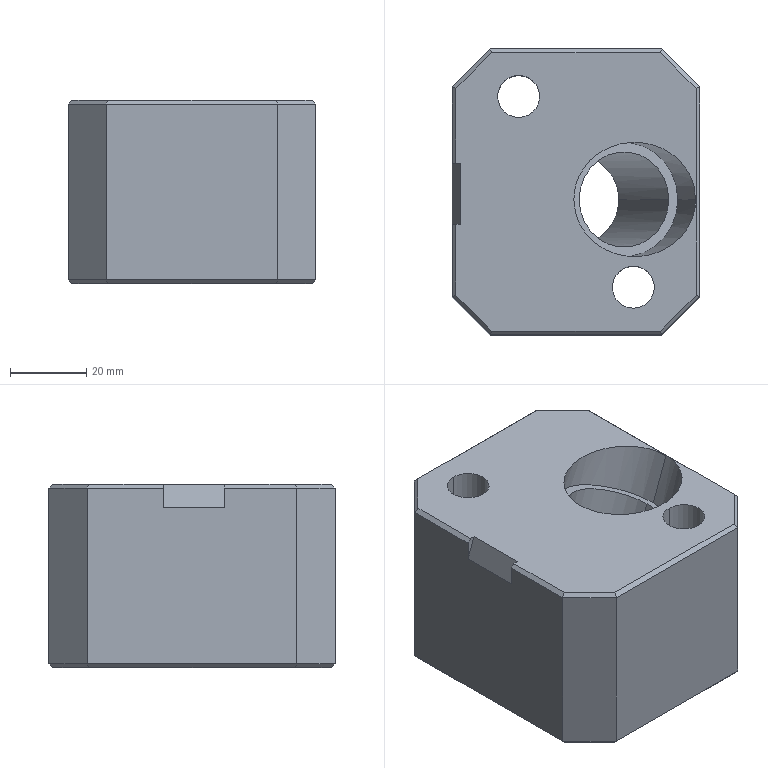Part | Creo | 1 solid | 49 faces | box 65 x 75 x 48 mm | volume 184557 mm3 | plane 33 | cylinder 16 | commonest cylinder face diameters 11 x4 18 x4 11.98 x2 12 x2 25 x2 30 x2
STEP:
#1=CARTESIAN_POINT('',(-250.936,-112.003,0.9999));
#2=VERTEX_POINT('',#1);
#3=CARTESIAN_POINT('',(-250.936,-94.003,0.9999));
#4=VERTEX_POINT('',#3);
#5=CARTESIAN_POINT('',(-250.936,-103.003,0.9999));
#6=DIRECTION('',(0.,0.,-1.));
#7=DIRECTION('',(0.,-1.,0.));
#8=AXIS2_PLACEMENT_3D('',#5,#6,#7);
#9=CIRCLE('',#8,9.);
#10=EDGE_CURVE('',#2,#4,#9,.T.);
#11=ORIENTED_EDGE('',*,*,#10,.F.);
#12=CARTESIAN_POINT('',(-250.936,-103.003,0.9999));
#13=DIRECTION('',(0.,0.,-1.));
#14=DIRECTION('',(0.,1.,0.));
#15=AXIS2_PLACEMENT_3D('',#12,#13,#14);
#16=CIRCLE('',#15,9.);
#17=EDGE_CURVE('',#4,#2,#16,.T.);
#18=ORIENTED_EDGE('',*,*,#17,.F.);
#19=EDGE_LOOP('',(#11,#18));
#20=FACE_OUTER_BOUND('',#19,.F.);
#21=CARTESIAN_POINT('',(-250.936,-108.503,0.9999));
#22=VERTEX_POINT('',#21);
#23=CARTESIAN_POINT('',(-250.936,-97.503,0.9999));
#24=VERTEX_POINT('',#23);
#25=CARTESIAN_POINT('',(-250.936,-103.003,1.));
#26=DIRECTION('',(0.,0.,1.));
#27=DIRECTION('',(0.,-1.,0.));
#28=AXIS2_PLACEMENT_3D('',#25,#26,#27);
#29=CIRCLE('',#28,5.5);
#30=EDGE_CURVE('',#22,#24,#29,.T.);
#31=ORIENTED_EDGE('',*,*,#30,.F.);
#32=CARTESIAN_POINT('',(-250.936,-103.003,1.));
#33=DIRECTION('',(0.,0.,1.));
#34=DIRECTION('',(0.,1.,0.));
#35=AXIS2_PLACEMENT_3D('',#32,#33,#34);
#36=CIRCLE('',#35,5.5);
#37=EDGE_CURVE('',#24,#22,#36,.T.);
#38=ORIENTED_EDGE('',*,*,#37,.F.);
#39=EDGE_LOOP('',(#31,#38));
#40=FACE_BOUND('',#39,.F.);
#41=CARTESIAN_POINT('',(-250.936,-94.253,1.));
#42=DIRECTION('',(0.,0.,1.));
#43=DIRECTION('',(1.,0.,0.));
#44=AXIS2_PLACEMENT_3D('',#41,#42,#43);
#45=PLANE('',#44);
#46=ADVANCED_FACE('',(#20,#40),#45,.F.);
#47=ORIENTED_EDGE('',*,*,#10,.T.);
#48=CARTESIAN_POINT('',(-250.936,-94.003,-10.));
#49=VERTEX_POINT('',#48);
#50=CARTESIAN_POINT('',(-250.936,-94.003,-10.));
#51=DIRECTION('',(0.,0.,1.));
#52=VECTOR('',#51,11.);
#53=LINE('',#50,#52);
#54=EDGE_CURVE('',#49,#4,#53,.T.);
#55=ORIENTED_EDGE('',*,*,#54,.F.);
#56=CARTESIAN_POINT('',(-250.936,-112.003,-10.));
#57=VERTEX_POINT('',#56);
#58=CARTESIAN_POINT('',(-250.936,-103.003,-10.));
#59=DIRECTION('',(0.,0.,1.));
#60=DIRECTION('',(0.,1.,0.));
#61=AXIS2_PLACEMENT_3D('',#58,#59,#60);
#62=CIRCLE('',#61,9.);
#63=EDGE_CURVE('',#49,#57,#62,.T.);
#64=ORIENTED_EDGE('',*,*,#63,.T.);
#65=CARTESIAN_POINT('',(-250.936,-112.003,-10.));
#66=DIRECTION('',(0.,0.,1.));
#67=VECTOR('',#66,11.);
#68=LINE('',#65,#67);
#69=EDGE_CURVE('',#57,#2,#68,.T.);
#70=ORIENTED_EDGE('',*,*,#69,.T.);
#71=EDGE_LOOP('',(#47,#55,#64,#70));
#72=FACE_OUTER_BOUND('',#71,.F.);
#73=CARTESIAN_POINT('',(-250.936,-103.003,-10.));
#74=DIRECTION('',(0.,0.,1.));
#75=DIRECTION('',(0.,-1.,0.));
#76=AXIS2_PLACEMENT_3D('',#73,#74,#75);
#77=CYLINDRICAL_SURFACE('',#76,9.);
#78=ADVANCED_FACE('',(#72),#77,.F.);
#79=ORIENTED_EDGE('',*,*,#17,.T.);
#80=ORIENTED_EDGE('',*,*,#69,.F.);
#81=CARTESIAN_POINT('',(-250.936,-103.003,-10.));
#82=DIRECTION('',(0.,0.,1.));
#83=DIRECTION('',(0.,-1.,0.));
#84=AXIS2_PLACEMENT_3D('',#81,#82,#83);
#85=CIRCLE('',#84,9.);
#86=EDGE_CURVE('',#57,#49,#85,.T.);
#87=ORIENTED_EDGE('',*,*,#86,.T.);
#88=ORIENTED_EDGE('',*,*,#54,.T.);
#89=EDGE_LOOP('',(#79,#80,#87,#88));
#90=FACE_OUTER_BOUND('',#89,.F.);
#91=CARTESIAN_POINT('',(-250.936,-103.003,-10.));
#92=DIRECTION('',(0.,0.,1.));
#93=DIRECTION('',(0.,-1.,0.));
#94=AXIS2_PLACEMENT_3D('',#91,#92,#93);
#95=CYLINDRICAL_SURFACE('',#94,9.);
#96=ADVANCED_FACE('',(#90),#95,.F.);
#97=CARTESIAN_POINT('',(-213.85,-91.503,-10.));
#98=VERTEX_POINT('',#97);
#99=CARTESIAN_POINT('',(-204.436,-100.917,-10.));
#100=VERTEX_POINT('',#99);
#101=CARTESIAN_POINT('',(-213.85,-91.503,-10.));
#102=DIRECTION('',(0.7071,-0.7071,0.));
#103=VECTOR('',#102,13.314);
#104=LINE('',#101,#103);
#105=EDGE_CURVE('',#98,#100,#104,.T.);
#106=ORIENTED_EDGE('',*,*,#105,.F.);
#107=CARTESIAN_POINT('',(-258.022,-91.503,-10.));
#108=VERTEX_POINT('',#107);
#109=CARTESIAN_POINT('',(-213.85,-91.503,-10.));
#110=DIRECTION('',(-1.,0.,0.));
#111=VECTOR('',#110,44.172);
#112=LINE('',#109,#111);
#113=EDGE_CURVE('',#98,#108,#112,.T.);
#114=ORIENTED_EDGE('',*,*,#113,.T.);
#115=CARTESIAN_POINT('',(-267.436,-100.917,-10.));
#116=VERTEX_POINT('',#115);
#117=CARTESIAN_POINT('',(-267.436,-100.917,-10.));
#118=DIRECTION('',(0.7071,0.7071,0.));
#119=VECTOR('',#118,13.314);
#120=LINE('',#117,#119);
#121=EDGE_CURVE('',#116,#108,#120,.T.);
#122=ORIENTED_EDGE('',*,*,#121,.F.);
#123=CARTESIAN_POINT('',(-267.436,-155.089,-10.));
#124=VERTEX_POINT('',#123);
#125=CARTESIAN_POINT('',(-267.436,-100.917,-10.));
#126=DIRECTION('',(0.,-1.,0.));
#127=VECTOR('',#126,54.172);
#128=LINE('',#125,#127);
#129=EDGE_CURVE('',#116,#124,#128,.T.);
#130=ORIENTED_EDGE('',*,*,#129,.T.);
#131=CARTESIAN_POINT('',(-258.022,-164.503,-10.));
#132=VERTEX_POINT('',#131);
#133=CARTESIAN_POINT('',(-258.022,-164.503,-10.));
#134=DIRECTION('',(-0.7071,0.7071,0.));
#135=VECTOR('',#134,13.314);
#136=LINE('',#133,#135);
#137=EDGE_CURVE('',#132,#124,#136,.T.);
#138=ORIENTED_EDGE('',*,*,#137,.F.);
#139=CARTESIAN_POINT('',(-213.85,-164.503,-10.));
#140=VERTEX_POINT('',#139);
#141=CARTESIAN_POINT('',(-258.022,-164.503,-10.));
#142=DIRECTION('',(1.,0.,0.));
#143=VECTOR('',#142,44.172);
#144=LINE('',#141,#143);
#145=EDGE_CURVE('',#132,#140,#144,.T.);
#146=ORIENTED_EDGE('',*,*,#145,.T.);
#147=CARTESIAN_POINT('',(-204.436,-155.089,-10.));
#148=VERTEX_POINT('',#147);
#149=CARTESIAN_POINT('',(-204.436,-155.089,-10.));
#150=DIRECTION('',(-0.7071,-0.7071,0.));
#151=VECTOR('',#150,13.314);
#152=LINE('',#149,#151);
#153=EDGE_CURVE('',#148,#140,#152,.T.);
#154=ORIENTED_EDGE('',*,*,#153,.F.);
#155=CARTESIAN_POINT('',(-204.436,-155.089,-10.));
#156=DIRECTION('',(0.,1.,0.));
#157=VECTOR('',#156,54.172);
#158=LINE('',#155,#157);
#159=EDGE_CURVE('',#148,#100,#158,.T.);
#160=ORIENTED_EDGE('',*,*,#159,.T.);
#161=EDGE_LOOP('',(#106,#114,#122,#130,#138,#146,#154,#160));
#162=FACE_OUTER_BOUND('',#161,.F.);
#163=CARTESIAN_POINT('',(-224.707,-130.005,-10.));
#164=VERTEX_POINT('',#163);
#165=CARTESIAN_POINT('',(-251.311,-130.005,-10.));
#166=VERTEX_POINT('',#165);
#167=CARTESIAN_POINT('',(-224.707,-130.005,-10.));
#168=CARTESIAN_POINT('',(-224.707,-131.478,-10.));
#169=CARTESIAN_POINT('',(-225.275,-134.662,-10.));
#170=CARTESIAN_POINT('',(-227.815,-138.362,-10.));
#171=CARTESIAN_POINT('',(-230.687,-140.546,-10.));
#172=CARTESIAN_POINT('',(-233.098,-141.711,-10.));
#173=CARTESIAN_POINT('',(-235.181,-142.263,-10.));
#174=CARTESIAN_POINT('',(-236.821,-142.472,-10.));
#175=CARTESIAN_POINT('',(-238.009,-142.521,-10.));
#176=CARTESIAN_POINT('',(-239.198,-142.472,-10.));
#177=CARTESIAN_POINT('',(-240.838,-142.263,-10.));
#178=CARTESIAN_POINT('',(-242.921,-141.711,-10.));
#179=CARTESIAN_POINT('',(-245.331,-140.546,-10.));
#180=CARTESIAN_POINT('',(-248.203,-138.362,-10.));
#181=CARTESIAN_POINT('',(-250.743,-134.662,-10.));
#182=CARTESIAN_POINT('',(-251.311,-131.478,-10.));
#183=CARTESIAN_POINT('',(-251.311,-130.005,-10.));
#184=B_SPLINE_CURVE_WITH_KNOTS('',3,(#167,#168,#169,#170,#171,#172,#173,#174,#175,#176,#177,#178,#179,#180,#181,#182,#183),.UNSPECIFIED.,.F.,.F.,(4,1,1,1,1,1,1,1,1,1,1,1,1,1,4),(0.,0.125,0.25,0.3125,0.375,0.4375,0.4688,0.5,0.5312,0.5625,0.625,0.6875,0.75,0.875,1.),.UNSPECIFIED.);
#185=EDGE_CURVE('',#164,#166,#184,.T.);
#186=ORIENTED_EDGE('',*,*,#185,.T.);
#187=CARTESIAN_POINT('',(-251.311,-130.005,-10.));
#188=CARTESIAN_POINT('',(-251.311,-128.532,-10.));
#189=CARTESIAN_POINT('',(-250.743,-125.348,-10.));
#190=CARTESIAN_POINT('',(-248.203,-121.647,-10.));
#191=CARTESIAN_POINT('',(-245.331,-119.463,-10.));
#192=CARTESIAN_POINT('',(-242.921,-118.299,-10.));
#193=CARTESIAN_POINT('',(-240.838,-117.746,-10.));
#194=CARTESIAN_POINT('',(-239.198,-117.537,-10.));
#195=CARTESIAN_POINT('',(-238.009,-117.488,-10.));
#196=CARTESIAN_POINT('',(-236.821,-117.537,-10.));
#197=CARTESIAN_POINT('',(-235.181,-117.746,-10.));
#198=CARTESIAN_POINT('',(-233.098,-118.299,-10.));
#199=CARTESIAN_POINT('',(-230.687,-119.463,-10.));
#200=CARTESIAN_POINT('',(-227.815,-121.647,-10.));
#201=CARTESIAN_POINT('',(-225.275,-125.348,-10.));
#202=CARTESIAN_POINT('',(-224.707,-128.532,-10.));
#203=CARTESIAN_POINT('',(-224.707,-130.005,-10.));
#204=B_SPLINE_CURVE_WITH_KNOTS('',3,(#187,#188,#189,#190,#191,#192,#193,#194,#195,#196,#197,#198,#199,#200,#201,#202,#203),.UNSPECIFIED.,.F.,.F.,(4,1,1,1,1,1,1,1,1,1,1,1,1,1,4),(0.,0.125,0.25,0.3125,0.375,0.4375,0.4688,0.5,0.5312,0.5625,0.625,0.6875,0.75,0.875,1.),.UNSPECIFIED.);
#205=EDGE_CURVE('',#166,#164,#204,.T.);
#206=ORIENTED_EDGE('',*,*,#205,.T.);
#207=EDGE_LOOP('',(#186,#206));
#208=FACE_BOUND('',#207,.F.);
#209=ORIENTED_EDGE('',*,*,#86,.F.);
#210=ORIENTED_EDGE('',*,*,#63,.F.);
#211=EDGE_LOOP('',(#209,#210));
#212=FACE_BOUND('',#211,.F.);
#213=CARTESIAN_POINT('',(-220.936,-162.003,-10.));
#214=VERTEX_POINT('',#213);
#215=CARTESIAN_POINT('',(-220.936,-144.003,-10.));
#216=VERTEX_POINT('',#215);
#217=CARTESIAN_POINT('',(-220.936,-153.003,-10.));
#218=DIRECTION('',(0.,0.,1.));
#219=DIRECTION('',(0.,-1.,0.));
#220=AXIS2_PLACEMENT_3D('',#217,#218,#219);
#221=CIRCLE('',#220,9.);
#222=EDGE_CURVE('',#214,#216,#221,.T.);
#223=ORIENTED_EDGE('',*,*,#222,.F.);
#224=CARTESIAN_POINT('',(-220.936,-153.003,-10.));
#225=DIRECTION('',(0.,0.,1.));
#226=DIRECTION('',(0.,1.,0.));
#227=AXIS2_PLACEMENT_3D('',#224,#225,#226);
#228=CIRCLE('',#227,9.);
#229=EDGE_CURVE('',#216,#214,#228,.T.);
#230=ORIENTED_EDGE('',*,*,#229,.F.);
#231=EDGE_LOOP('',(#223,#230));
#232=FACE_BOUND('',#231,.F.);
#233=CARTESIAN_POINT('',(605.564,-97.003,-10.));
#234=DIRECTION('',(0.,0.,1.));
#235=DIRECTION('',(-1.,0.,0.));
#236=AXIS2_PLACEMENT_3D('',#233,#234,#235);
#237=PLANE('',#236);
#238=ADVANCED_FACE('',(#162,#208,#212,#232),#237,.F.);
#239=CARTESIAN_POINT('',(-211.613,-130.005,25.977));
#240=VERTEX_POINT('',#239);
#241=CARTESIAN_POINT('',(-235.105,-130.005,34.527));
#242=VERTEX_POINT('',#241);
#243=CARTESIAN_POINT('',(-223.359,-130.005,30.252));
#244=DIRECTION('',(-0.342,0.,-0.9397));
#245=DIRECTION('',(0.9397,0.,-0.342));
#246=AXIS2_PLACEMENT_3D('',#243,#244,#245);
#247=CIRCLE('',#246,12.5);
#248=EDGE_CURVE('',#240,#242,#247,.T.);
#249=ORIENTED_EDGE('',*,*,#248,.T.);
#250=CARTESIAN_POINT('',(-235.105,-130.005,34.527));
#251=DIRECTION('',(-0.342,0.,-0.9397));
#252=VECTOR('',#251,47.385);
#253=LINE('',#250,#252);
#254=EDGE_CURVE('',#242,#166,#253,.T.);
#255=ORIENTED_EDGE('',*,*,#254,.T.);
#256=ORIENTED_EDGE('',*,*,#185,.F.);
#257=CARTESIAN_POINT('',(-211.613,-130.005,25.977));
#258=DIRECTION('',(-0.342,0.,-0.9397));
#259=VECTOR('',#258,38.286);
#260=LINE('',#257,#259);
#261=EDGE_CURVE('',#240,#164,#260,.T.);
#262=ORIENTED_EDGE('',*,*,#261,.F.);
#263=EDGE_LOOP('',(#249,#255,#256,#262));
#264=FACE_OUTER_BOUND('',#263,.F.);
#265=CARTESIAN_POINT('',(-211.802,-130.005,62.004));
#266=DIRECTION('',(-0.342,0.,-0.9397));
#267=DIRECTION('',(-0.9397,0.,0.342));
#268=AXIS2_PLACEMENT_3D('',#265,#266,#267);
#269=CYLINDRICAL_SURFACE('',#268,12.5);
#270=ADVANCED_FACE('',(#264),#269,.F.);
#271=CARTESIAN_POINT('',(-209.263,-130.005,25.122));
#272=VERTEX_POINT('',#271);
#273=CARTESIAN_POINT('',(-237.454,-130.005,35.382));
#274=VERTEX_POINT('',#273);
#275=CARTESIAN_POINT('',(-223.359,-130.005,30.252));
#276=DIRECTION('',(0.342,0.,0.9397));
#277=DIRECTION('',(0.9397,0.,-0.342));
#278=AXIS2_PLACEMENT_3D('',#275,#276,#277);
#279=CIRCLE('',#278,15.);
#280=EDGE_CURVE('',#272,#274,#279,.T.);
#281=ORIENTED_EDGE('',*,*,#280,.F.);
#282=CARTESIAN_POINT('',(-223.359,-130.005,30.252));
#283=DIRECTION('',(0.342,0.,0.9397));
#284=DIRECTION('',(-0.9397,0.,0.342));
#285=AXIS2_PLACEMENT_3D('',#282,#283,#284);
#286=CIRCLE('',#285,15.);
#287=EDGE_CURVE('',#274,#272,#286,.T.);
#288=ORIENTED_EDGE('',*,*,#287,.F.);
#289=EDGE_LOOP('',(#281,#288));
#290=FACE_OUTER_BOUND('',#289,.F.);
#291=ORIENTED_EDGE('',*,*,#248,.F.);
#292=CARTESIAN_POINT('',(-223.359,-130.005,30.252));
#293=DIRECTION('',(-0.342,0.,-0.9397));
#294=DIRECTION('',(-0.9397,0.,0.342));
#295=AXIS2_PLACEMENT_3D('',#292,#293,#294);
#296=CIRCLE('',#295,12.5);
#297=EDGE_CURVE('',#242,#240,#296,.T.);
#298=ORIENTED_EDGE('',*,*,#297,.F.);
#299=EDGE_LOOP('',(#291,#298));
#300=FACE_BOUND('',#299,.F.);
#301=CARTESIAN_POINT('',(-223.359,-130.005,30.252));
#302=DIRECTION('',(-0.342,0.,-0.9397));
#303=DIRECTION('',(-0.9397,0.,0.342));
#304=AXIS2_PLACEMENT_3D('',#301,#302,#303);
#305=PLANE('',#304);
#306=ADVANCED_FACE('',(#290,#300),#305,.F.);
#307=ORIENTED_EDGE('',*,*,#297,.T.);
#308=ORIENTED_EDGE('',*,*,#261,.T.);
#309=ORIENTED_EDGE('',*,*,#205,.F.);
#310=ORIENTED_EDGE('',*,*,#254,.F.);
#311=EDGE_LOOP('',(#307,#308,#309,#310));
#312=FACE_OUTER_BOUND('',#311,.F.);
#313=CARTESIAN_POINT('',(-211.802,-130.005,62.004));
#314=DIRECTION('',(-0.342,0.,-0.9397));
#315=DIRECTION('',(-0.9397,0.,0.342));
#316=AXIS2_PLACEMENT_3D('',#313,#314,#315);
#317=CYLINDRICAL_SURFACE('',#316,12.5);
#318=ADVANCED_FACE('',(#312),#317,.F.);
#319=CARTESIAN_POINT('',(-204.576,-130.005,38.));
#320=VERTEX_POINT('',#319);
#321=CARTESIAN_POINT('',(-236.501,-130.005,38.));
#322=VERTEX_POINT('',#321);
#323=CARTESIAN_POINT('',(-204.576,-130.005,38.));
#324=CARTESIAN_POINT('',(-204.576,-128.237,38.));
#325=CARTESIAN_POINT('',(-205.258,-124.416,38.));
#326=CARTESIAN_POINT('',(-208.306,-119.975,38.));
#327=CARTESIAN_POINT('',(-211.753,-117.355,38.));
#328=CARTESIAN_POINT('',(-214.645,-115.958,38.));
#329=CARTESIAN_POINT('',(-217.145,-115.294,38.));
#330=CARTESIAN_POINT('',(-219.113,-115.044,38.));
#331=CARTESIAN_POINT('',(-220.539,-114.985,38.));
#332=CARTESIAN_POINT('',(-221.965,-115.044,38.));
#333=CARTESIAN_POINT('',(-223.933,-115.294,38.));
#334=CARTESIAN_POINT('',(-226.432,-115.958,38.));
#335=CARTESIAN_POINT('',(-229.325,-117.355,38.));
#336=CARTESIAN_POINT('',(-232.772,-119.975,38.));
#337=CARTESIAN_POINT('',(-235.82,-124.416,38.));
#338=CARTESIAN_POINT('',(-236.501,-128.237,38.));
#339=CARTESIAN_POINT('',(-236.501,-130.005,38.));
#340=B_SPLINE_CURVE_WITH_KNOTS('',3,(#323,#324,#325,#326,#327,#328,#329,#330,#331,#332,#333,#334,#335,#336,#337,#338,#339),.UNSPECIFIED.,.F.,.F.,(4,1,1,1,1,1,1,1,1,1,1,1,1,1,4),(0.,0.125,0.25,0.3125,0.375,0.4375,0.4688,0.5,0.5312,0.5625,0.625,0.6875,0.75,0.875,1.),.UNSPECIFIED.);
#341=EDGE_CURVE('',#320,#322,#340,.T.);
#342=ORIENTED_EDGE('',*,*,#341,.F.);
#343=CARTESIAN_POINT('',(-204.576,-130.005,38.));
#344=DIRECTION('',(-0.342,0.,-0.9397));
#345=VECTOR('',#344,13.705);
#346=LINE('',#343,#345);
#347=EDGE_CURVE('',#320,#272,#346,.T.);
#348=ORIENTED_EDGE('',*,*,#347,.T.);
#349=ORIENTED_EDGE('',*,*,#280,.T.);
#350=CARTESIAN_POINT('',(-236.501,-130.005,38.));
#351=DIRECTION('',(-0.342,0.,-0.9397));
#352=VECTOR('',#351,2.786);
#353=LINE('',#350,#352);
#354=EDGE_CURVE('',#322,#274,#353,.T.);
#355=ORIENTED_EDGE('',*,*,#354,.F.);
#356=EDGE_LOOP('',(#342,#348,#349,#355));
#357=FACE_OUTER_BOUND('',#356,.F.);
#358=CARTESIAN_POINT('',(-217.527,-130.005,46.274));
#359=DIRECTION('',(-0.342,0.,-0.9397));
#360=DIRECTION('',(-0.9397,0.,0.342));
#361=AXIS2_PLACEMENT_3D('',#358,#359,#360);
#362=CYLINDRICAL_SURFACE('',#361,15.);
#363=ADVANCED_FACE('',(#357),#362,.F.);
#364=CARTESIAN_POINT('',(-266.228,-136.503,38.));
#365=VERTEX_POINT('',#364);
#366=CARTESIAN_POINT('',(-267.436,-136.503,38.));
#367=VERTEX_POINT('',#366);
#368=CARTESIAN_POINT('',(-266.228,-136.503,38.));
#369=DIRECTION('',(-1.,0.,0.));
#370=VECTOR('',#369,1.208);
#371=LINE('',#368,#370);
#372=EDGE_CURVE('',#365,#367,#371,.T.);
#373=ORIENTED_EDGE('',*,*,#372,.F.);
#374=CARTESIAN_POINT('',(-266.228,-120.503,38.));
#375=VERTEX_POINT('',#374);
#376=CARTESIAN_POINT('',(-266.228,-120.503,38.));
#377=DIRECTION('',(0.,-1.,0.));
#378=VECTOR('',#377,16.);
#379=LINE('',#376,#378);
#380=EDGE_CURVE('',#375,#365,#379,.T.);
#381=ORIENTED_EDGE('',*,*,#380,.F.);
#382=CARTESIAN_POINT('',(-267.436,-120.503,38.));
#383=VERTEX_POINT('',#382);
#384=CARTESIAN_POINT('',(-267.436,-120.503,38.));
#385=DIRECTION('',(1.,0.,0.));
#386=VECTOR('',#385,1.208);
#387=LINE('',#384,#386);
#388=EDGE_CURVE('',#383,#375,#387,.T.);
#389=ORIENTED_EDGE('',*,*,#388,.F.);
#390=CARTESIAN_POINT('',(-267.436,-100.917,38.));
#391=VERTEX_POINT('',#390);
#392=CARTESIAN_POINT('',(-267.436,-120.503,38.));
#393=DIRECTION('',(0.,1.,0.));
#394=VECTOR('',#393,19.586);
#395=LINE('',#392,#394);
#396=EDGE_CURVE('',#383,#391,#395,.T.);
#397=ORIENTED_EDGE('',*,*,#396,.T.);
#398=CARTESIAN_POINT('',(-258.022,-91.503,38.));
#399=VERTEX_POINT('',#398);
#400=CARTESIAN_POINT('',(-258.022,-91.503,38.));
#401=DIRECTION('',(-0.7071,-0.7071,0.));
#402=VECTOR('',#401,13.314);
#403=LINE('',#400,#402);
#404=EDGE_CURVE('',#399,#391,#403,.T.);
#405=ORIENTED_EDGE('',*,*,#404,.F.);
#406=CARTESIAN_POINT('',(-213.85,-91.503,38.));
#407=VERTEX_POINT('',#406);
#408=CARTESIAN_POINT('',(-258.022,-91.503,38.));
#409=DIRECTION('',(1.,0.,0.));
#410=VECTOR('',#409,44.172);
#411=LINE('',#408,#410);
#412=EDGE_CURVE('',#399,#407,#411,.T.);
#413=ORIENTED_EDGE('',*,*,#412,.T.);
#414=CARTESIAN_POINT('',(-204.436,-100.917,38.));
#415=VERTEX_POINT('',#414);
#416=CARTESIAN_POINT('',(-204.436,-100.917,38.));
#417=DIRECTION('',(-0.7071,0.7071,0.));
#418=VECTOR('',#417,13.314);
#419=LINE('',#416,#418);
#420=EDGE_CURVE('',#415,#407,#419,.T.);
#421=ORIENTED_EDGE('',*,*,#420,.F.);
#422=CARTESIAN_POINT('',(-204.436,-155.089,38.));
#423=VERTEX_POINT('',#422);
#424=CARTESIAN_POINT('',(-204.436,-100.917,38.));
#425=DIRECTION('',(0.,-1.,0.));
#426=VECTOR('',#425,54.172);
#427=LINE('',#424,#426);
#428=EDGE_CURVE('',#415,#423,#427,.T.);
#429=ORIENTED_EDGE('',*,*,#428,.T.);
#430=CARTESIAN_POINT('',(-213.85,-164.503,38.));
#431=VERTEX_POINT('',#430);
#432=CARTESIAN_POINT('',(-213.85,-164.503,38.));
#433=DIRECTION('',(0.7071,0.7071,0.));
#434=VECTOR('',#433,13.314);
#435=LINE('',#432,#434);
#436=EDGE_CURVE('',#431,#423,#435,.T.);
#437=ORIENTED_EDGE('',*,*,#436,.F.);
#438=CARTESIAN_POINT('',(-258.022,-164.503,38.));
#439=VERTEX_POINT('',#438);
#440=CARTESIAN_POINT('',(-213.85,-164.503,38.));
#441=DIRECTION('',(-1.,0.,0.));
#442=VECTOR('',#441,44.172);
#443=LINE('',#440,#442);
#444=EDGE_CURVE('',#431,#439,#443,.T.);
#445=ORIENTED_EDGE('',*,*,#444,.T.);
#446=CARTESIAN_POINT('',(-267.436,-155.089,38.));
#447=VERTEX_POINT('',#446);
#448=CARTESIAN_POINT('',(-267.436,-155.089,38.));
#449=DIRECTION('',(0.7071,-0.7071,0.));
#450=VECTOR('',#449,13.314);
#451=LINE('',#448,#450);
#452=EDGE_CURVE('',#447,#439,#451,.T.);
#453=ORIENTED_EDGE('',*,*,#452,.F.);
#454=CARTESIAN_POINT('',(-267.436,-155.089,38.));
#455=DIRECTION('',(0.,1.,0.));
#456=VECTOR('',#455,18.586);
#457=LINE('',#454,#456);
#458=EDGE_CURVE('',#447,#367,#457,.T.);
#459=ORIENTED_EDGE('',*,*,#458,.T.);
#460=EDGE_LOOP('',(#373,#381,#389,#397,#405,#413,#421,#429,#437,#445,#453,#459));
#461=FACE_OUTER_BOUND('',#460,.F.);
#462=CARTESIAN_POINT('',(-250.936,-108.503,38.));
#463=VERTEX_POINT('',#462);
#464=CARTESIAN_POINT('',(-250.936,-97.503,38.));
#465=VERTEX_POINT('',#464);
#466=CARTESIAN_POINT('',(-250.936,-103.003,38.));
#467=DIRECTION('',(0.,0.,-1.));
#468=DIRECTION('',(0.,-1.,0.));
#469=AXIS2_PLACEMENT_3D('',#466,#467,#468);
#470=CIRCLE('',#469,5.5);
#471=EDGE_CURVE('',#463,#465,#470,.T.);
#472=ORIENTED_EDGE('',*,*,#471,.F.);
#473=CARTESIAN_POINT('',(-250.936,-103.003,38.));
#474=DIRECTION('',(0.,0.,-1.));
#475=DIRECTION('',(0.,1.,0.));
#476=AXIS2_PLACEMENT_3D('',#473,#474,#475);
#477=CIRCLE('',#476,5.5);
#478=EDGE_CURVE('',#465,#463,#477,.T.);
#479=ORIENTED_EDGE('',*,*,#478,.F.);
#480=EDGE_LOOP('',(#472,#479));
#481=FACE_BOUND('',#480,.F.);
#482=CARTESIAN_POINT('',(-220.936,-158.503,38.));
#483=VERTEX_POINT('',#482);
#484=CARTESIAN_POINT('',(-220.936,-147.503,38.));
#485=VERTEX_POINT('',#484);
#486=CARTESIAN_POINT('',(-220.936,-153.003,38.));
#487=DIRECTION('',(0.,0.,-1.));
#488=DIRECTION('',(0.,-1.,0.));
#489=AXIS2_PLACEMENT_3D('',#486,#487,#488);
#490=CIRCLE('',#489,5.5);
#491=EDGE_CURVE('',#483,#485,#490,.T.);
#492=ORIENTED_EDGE('',*,*,#491,.F.);
#493=CARTESIAN_POINT('',(-220.936,-153.003,38.));
#494=DIRECTION('',(0.,0.,-1.));
#495=DIRECTION('',(0.,1.,0.));
#496=AXIS2_PLACEMENT_3D('',#493,#494,#495);
#497=CIRCLE('',#496,5.5);
#498=EDGE_CURVE('',#485,#483,#497,.T.);
#499=ORIENTED_EDGE('',*,*,#498,.F.);
#500=EDGE_LOOP('',(#492,#499));
#501=FACE_BOUND('',#500,.F.);
#502=ORIENTED_EDGE('',*,*,#341,.T.);
#503=CARTESIAN_POINT('',(-236.501,-130.005,38.));
#504=CARTESIAN_POINT('',(-236.501,-131.772,38.));
#505=CARTESIAN_POINT('',(-235.82,-135.593,38.));
#506=CARTESIAN_POINT('',(-232.772,-140.034,38.));
#507=CARTESIAN_POINT('',(-229.325,-142.654,38.));
#508=CARTESIAN_POINT('',(-226.432,-144.052,38.));
#509=CARTESIAN_POINT('',(-223.933,-144.715,38.));
#510=CARTESIAN_POINT('',(-221.965,-144.966,38.));
#511=CARTESIAN_POINT('',(-220.539,-145.024,38.));
#512=CARTESIAN_POINT('',(-219.113,-144.966,38.));
#513=CARTESIAN_POINT('',(-217.145,-144.715,38.));
#514=CARTESIAN_POINT('',(-214.645,-144.052,38.));
#515=CARTESIAN_POINT('',(-211.753,-142.654,38.));
#516=CARTESIAN_POINT('',(-208.306,-140.034,38.));
#517=CARTESIAN_POINT('',(-205.258,-135.593,38.));
#518=CARTESIAN_POINT('',(-204.576,-131.772,38.));
#519=CARTESIAN_POINT('',(-204.576,-130.005,38.));
#520=B_SPLINE_CURVE_WITH_KNOTS('',3,(#503,#504,#505,#506,#507,#508,#509,#510,#511,#512,#513,#514,#515,#516,#517,#518,#519),.UNSPECIFIED.,.F.,.F.,(4,1,1,1,1,1,1,1,1,1,1,1,1,1,4),(0.,0.125,0.25,0.3125,0.375,0.4375,0.4688,0.5,0.5312,0.5625,0.625,0.6875,0.75,0.875,1.),.UNSPECIFIED.);
#521=EDGE_CURVE('',#322,#320,#520,.T.);
#522=ORIENTED_EDGE('',*,*,#521,.T.);
#523=EDGE_LOOP('',(#502,#522));
#524=FACE_BOUND('',#523,.F.);
#525=CARTESIAN_POINT('',(-222.833,-493.939,38.));
#526=DIRECTION('',(0.,0.,1.));
#527=DIRECTION('',(0.,1.,0.));
#528=AXIS2_PLACEMENT_3D('',#525,#526,#527);
#529=PLANE('',#528);
#530=ADVANCED_FACE('',(#461,#481,#501,#524),#529,.T.);
#531=ORIENTED_EDGE('',*,*,#372,.T.);
#532=CARTESIAN_POINT('',(-268.436,-136.503,37.));
#533=VERTEX_POINT('',#532);
#534=CARTESIAN_POINT('',(-268.436,-136.503,37.));
#535=DIRECTION('',(0.7071,0.,0.7071));
#536=VECTOR('',#535,1.414);
#537=LINE('',#534,#536);
#538=EDGE_CURVE('',#533,#367,#537,.T.);
#539=ORIENTED_EDGE('',*,*,#538,.F.);
#540=CARTESIAN_POINT('',(-268.436,-136.503,31.933));
#541=VERTEX_POINT('',#540);
#542=CARTESIAN_POINT('',(-268.436,-136.503,37.));
#543=DIRECTION('',(0.,0.,-1.));
#544=VECTOR('',#543,5.067);
#545=LINE('',#542,#544);
#546=EDGE_CURVE('',#533,#541,#545,.T.);
#547=ORIENTED_EDGE('',*,*,#546,.T.);
#548=CARTESIAN_POINT('',(-266.228,-136.503,38.));
#549=DIRECTION('',(-0.342,0.,-0.9397));
#550=VECTOR('',#549,6.456);
#551=LINE('',#548,#550);
#552=EDGE_CURVE('',#365,#541,#551,.T.);
#553=ORIENTED_EDGE('',*,*,#552,.F.);
#554=EDGE_LOOP('',(#531,#539,#547,#553));
#555=FACE_OUTER_BOUND('',#554,.F.);
#556=CARTESIAN_POINT('',(-285.225,-136.503,-2.889));
#557=DIRECTION('',(0.,-1.,0.));
#558=DIRECTION('',(0.,0.,-1.));
#559=AXIS2_PLACEMENT_3D('',#556,#557,#558);
#560=PLANE('',#559);
#561=ADVANCED_FACE('',(#555),#560,.F.);
#562=ORIENTED_EDGE('',*,*,#538,.T.);
#563=ORIENTED_EDGE('',*,*,#458,.F.);
#564=CARTESIAN_POINT('',(-268.436,-155.503,37.));
#565=VERTEX_POINT('',#564);
#566=CARTESIAN_POINT('',(-268.436,-155.503,37.));
#567=DIRECTION('',(0.6786,0.2811,0.6786));
#568=VECTOR('',#567,1.474);
#569=LINE('',#566,#568);
#570=EDGE_CURVE('',#565,#447,#569,.T.);
#571=ORIENTED_EDGE('',*,*,#570,.F.);
#572=CARTESIAN_POINT('',(-268.436,-136.503,37.));
#573=DIRECTION('',(0.,-1.,0.));
#574=VECTOR('',#573,19.);
#575=LINE('',#572,#574);
#576=EDGE_CURVE('',#533,#565,#575,.T.);
#577=ORIENTED_EDGE('',*,*,#576,.F.);
#578=EDGE_LOOP('',(#562,#563,#571,#577));
#579=FACE_OUTER_BOUND('',#578,.F.);
#580=CARTESIAN_POINT('',(-267.436,-493.939,38.));
#581=DIRECTION('',(0.7071,0.,-0.7071));
#582=DIRECTION('',(0.,-1.,0.));
#583=AXIS2_PLACEMENT_3D('',#580,#581,#582);
#584=PLANE('',#583);
#585=ADVANCED_FACE('',(#579),#584,.F.);
#586=ORIENTED_EDGE('',*,*,#452,.T.);
#587=CARTESIAN_POINT('',(-258.436,-165.503,37.));
#588=VERTEX_POINT('',#587);
#589=CARTESIAN_POINT('',(-258.436,-165.503,37.));
#590=DIRECTION('',(0.2811,0.6786,0.6786));
#591=VECTOR('',#590,1.474);
#592=LINE('',#589,#591);
#593=EDGE_CURVE('',#588,#439,#592,.T.);
#594=ORIENTED_EDGE('',*,*,#593,.F.);
#595=CARTESIAN_POINT('',(-268.436,-155.503,37.));
#596=DIRECTION('',(0.7071,-0.7071,0.));
#597=VECTOR('',#596,14.142);
#598=LINE('',#595,#597);
#599=EDGE_CURVE('',#565,#588,#598,.T.);
#600=ORIENTED_EDGE('',*,*,#599,.F.);
#601=ORIENTED_EDGE('',*,*,#570,.T.);
#602=EDGE_LOOP('',(#586,#594,#600,#601));
#603=FACE_OUTER_BOUND('',#602,.F.);
#604=CARTESIAN_POINT('',(-75.709,-346.815,38.));
#605=DIRECTION('',(0.5,0.5,-0.7071));
#606=DIRECTION('',(0.7071,-0.7071,0.));
#607=AXIS2_PLACEMENT_3D('',#604,#605,#606);
#608=PLANE('',#607);
#609=ADVANCED_FACE('',(#603),#608,.F.);
#610=ORIENTED_EDGE('',*,*,#593,.T.);
#611=ORIENTED_EDGE('',*,*,#444,.F.);
#612=CARTESIAN_POINT('',(-213.436,-165.503,37.));
#613=VERTEX_POINT('',#612);
#614=CARTESIAN_POINT('',(-213.436,-165.503,37.));
#615=DIRECTION('',(-0.2811,0.6786,0.6786));
#616=VECTOR('',#615,1.474);
#617=LINE('',#614,#616);
#618=EDGE_CURVE('',#613,#431,#617,.T.);
#619=ORIENTED_EDGE('',*,*,#618,.F.);
#620=CARTESIAN_POINT('',(-258.436,-165.503,37.));
#621=DIRECTION('',(1.,0.,0.));
#622=VECTOR('',#621,45.);
#623=LINE('',#620,#622);
#624=EDGE_CURVE('',#588,#613,#623,.T.);
#625=ORIENTED_EDGE('',*,*,#624,.F.);
#626=EDGE_LOOP('',(#610,#611,#619,#625));
#627=FACE_OUTER_BOUND('',#626,.F.);
#628=CARTESIAN_POINT('',(-222.833,-164.503,38.));
#629=DIRECTION('',(0.,-0.7071,0.7071));
#630=DIRECTION('',(-1.,0.,0.));
#631=AXIS2_PLACEMENT_3D('',#628,#629,#630);
#632=PLANE('',#631);
#633=ADVANCED_FACE('',(#627),#632,.T.);
#634=ORIENTED_EDGE('',*,*,#618,.T.);
#635=ORIENTED_EDGE('',*,*,#436,.T.);
#636=CARTESIAN_POINT('',(-203.436,-155.503,37.));
#637=VERTEX_POINT('',#636);
#638=CARTESIAN_POINT('',(-203.436,-155.503,37.));
#639=DIRECTION('',(-0.6786,0.2811,0.6786));
#640=VECTOR('',#639,1.474);
#641=LINE('',#638,#640);
#642=EDGE_CURVE('',#637,#423,#641,.T.);
#643=ORIENTED_EDGE('',*,*,#642,.F.);
#644=CARTESIAN_POINT('',(-213.436,-165.503,37.));
#645=DIRECTION('',(0.7071,0.7071,0.));
#646=VECTOR('',#645,14.142);
#647=LINE('',#644,#646);
#648=EDGE_CURVE('',#613,#637,#647,.T.);
#649=ORIENTED_EDGE('',*,*,#648,.F.);
#650=EDGE_LOOP('',(#634,#635,#643,#649));
#651=FACE_OUTER_BOUND('',#650,.F.);
#652=CARTESIAN_POINT('',(-383.06,-333.713,38.));
#653=DIRECTION('',(-0.5,0.5,-0.7071));
#654=DIRECTION('',(0.7071,0.7071,0.));
#655=AXIS2_PLACEMENT_3D('',#652,#653,#654);
#656=PLANE('',#655);
#657=ADVANCED_FACE('',(#651),#656,.F.);
#658=CARTESIAN_POINT('',(-203.436,-100.503,37.));
#659=VERTEX_POINT('',#658);
#660=CARTESIAN_POINT('',(-203.436,-100.503,37.));
#661=DIRECTION('',(-0.6786,-0.2811,0.6786));
#662=VECTOR('',#661,1.474);
#663=LINE('',#660,#662);
#664=EDGE_CURVE('',#659,#415,#663,.T.);
#665=ORIENTED_EDGE('',*,*,#664,.F.);
#666=CARTESIAN_POINT('',(-203.436,-155.503,37.));
#667=DIRECTION('',(0.,1.,0.));
#668=VECTOR('',#667,55.);
#669=LINE('',#666,#668);
#670=EDGE_CURVE('',#637,#659,#669,.T.);
#671=ORIENTED_EDGE('',*,*,#670,.F.);
#672=ORIENTED_EDGE('',*,*,#642,.T.);
#673=ORIENTED_EDGE('',*,*,#428,.F.);
#674=EDGE_LOOP('',(#665,#671,#672,#673));
#675=FACE_OUTER_BOUND('',#674,.F.);
#676=CARTESIAN_POINT('',(-203.436,-406.503,37.));
#677=DIRECTION('',(-0.7071,0.,-0.7071));
#678=DIRECTION('',(0.,-1.,0.));
#679=AXIS2_PLACEMENT_3D('',#676,#677,#678);
#680=PLANE('',#679);
#681=ADVANCED_FACE('',(#675),#680,.F.);
#682=ORIENTED_EDGE('',*,*,#664,.T.);
#683=ORIENTED_EDGE('',*,*,#420,.T.);
#684=CARTESIAN_POINT('',(-213.436,-90.503,37.));
#685=VERTEX_POINT('',#684);
#686=CARTESIAN_POINT('',(-213.85,-91.503,38.));
#687=DIRECTION('',(0.2811,0.6786,-0.6786));
#688=VECTOR('',#687,1.474);
#689=LINE('',#686,#688);
#690=EDGE_CURVE('',#407,#685,#689,.T.);
#691=ORIENTED_EDGE('',*,*,#690,.T.);
#692=CARTESIAN_POINT('',(-203.436,-100.503,37.));
#693=DIRECTION('',(-0.7071,0.7071,0.));
#694=VECTOR('',#693,14.142);
#695=LINE('',#692,#694);
#696=EDGE_CURVE('',#659,#685,#695,.T.);
#697=ORIENTED_EDGE('',*,*,#696,.F.);
#698=EDGE_LOOP('',(#682,#683,#691,#697));
#699=FACE_OUTER_BOUND('',#698,.F.);
#700=CARTESIAN_POINT('',(-17.124,-288.23,38.));
#701=DIRECTION('',(0.5,0.5,0.7071));
#702=DIRECTION('',(0.7071,-0.7071,0.));
#703=AXIS2_PLACEMENT_3D('',#700,#701,#702);
#704=PLANE('',#703);
#705=ADVANCED_FACE('',(#699),#704,.T.);
#706=CARTESIAN_POINT('',(-258.436,-90.503,37.));
#707=VERTEX_POINT('',#706);
#708=CARTESIAN_POINT('',(-258.022,-91.503,38.));
#709=DIRECTION('',(-0.2811,0.6786,-0.6786));
#710=VECTOR('',#709,1.474);
#711=LINE('',#708,#710);
#712=EDGE_CURVE('',#399,#707,#711,.T.);
#713=ORIENTED_EDGE('',*,*,#712,.T.);
#714=CARTESIAN_POINT('',(-213.436,-90.503,37.));
#715=DIRECTION('',(-1.,0.,0.));
#716=VECTOR('',#715,45.);
#717=LINE('',#714,#716);
#718=EDGE_CURVE('',#685,#707,#717,.T.);
#719=ORIENTED_EDGE('',*,*,#718,.F.);
#720=ORIENTED_EDGE('',*,*,#690,.F.);
#721=ORIENTED_EDGE('',*,*,#412,.F.);
#722=EDGE_LOOP('',(#713,#719,#720,#721));
#723=FACE_OUTER_BOUND('',#722,.F.);
#724=CARTESIAN_POINT('',(-222.833,-91.503,38.));
#725=DIRECTION('',(0.,-0.7071,-0.7071));
#726=DIRECTION('',(-1.,0.,0.));
#727=AXIS2_PLACEMENT_3D('',#724,#725,#726);
#728=PLANE('',#727);
#729=ADVANCED_FACE('',(#723),#728,.F.);
#730=CARTESIAN_POINT('',(-268.436,-100.503,37.));
#731=VERTEX_POINT('',#730);
#732=CARTESIAN_POINT('',(-258.436,-90.503,37.));
#733=DIRECTION('',(-0.7071,-0.7071,0.));
#734=VECTOR('',#733,14.142);
#735=LINE('',#732,#734);
#736=EDGE_CURVE('',#707,#731,#735,.T.);
#737=ORIENTED_EDGE('',*,*,#736,.F.);
#738=ORIENTED_EDGE('',*,*,#712,.F.);
#739=ORIENTED_EDGE('',*,*,#404,.T.);
#740=CARTESIAN_POINT('',(-267.436,-100.917,38.));
#741=DIRECTION('',(-0.6786,0.2811,-0.6786));
#742=VECTOR('',#741,1.474);
#743=LINE('',#740,#742);
#744=EDGE_CURVE('',#391,#731,#743,.T.);
#745=ORIENTED_EDGE('',*,*,#744,.T.);
#746=EDGE_LOOP('',(#737,#738,#739,#745));
#747=FACE_OUTER_BOUND('',#746,.F.);
#748=CARTESIAN_POINT('',(-441.645,-275.127,38.));
#749=DIRECTION('',(-0.5,0.5,0.7071));
#750=DIRECTION('',(0.7071,0.7071,0.));
#751=AXIS2_PLACEMENT_3D('',#748,#749,#750);
#752=PLANE('',#751);
#753=ADVANCED_FACE('',(#747),#752,.T.);
#754=CARTESIAN_POINT('',(-268.436,-100.503,-9.));
#755=VERTEX_POINT('',#754);
#756=CARTESIAN_POINT('',(-268.436,-100.503,-9.));
#757=DIRECTION('',(0.,0.,1.));
#758=VECTOR('',#757,46.);
#759=LINE('',#756,#758);
#760=EDGE_CURVE('',#755,#731,#759,.T.);
#761=ORIENTED_EDGE('',*,*,#760,.F.);
#762=CARTESIAN_POINT('',(-258.436,-90.503,-9.));
#763=VERTEX_POINT('',#762);
#764=CARTESIAN_POINT('',(-268.436,-100.503,-9.));
#765=DIRECTION('',(0.7071,0.7071,0.));
#766=VECTOR('',#765,14.142);
#767=LINE('',#764,#766);
#768=EDGE_CURVE('',#755,#763,#767,.T.);
#769=ORIENTED_EDGE('',*,*,#768,.T.);
#770=CARTESIAN_POINT('',(-258.436,-90.503,37.));
#771=DIRECTION('',(0.,0.,-1.));
#772=VECTOR('',#771,46.);
#773=LINE('',#770,#772);
#774=EDGE_CURVE('',#707,#763,#773,.T.);
#775=ORIENTED_EDGE('',*,*,#774,.F.);
#776=ORIENTED_EDGE('',*,*,#736,.T.);
#777=EDGE_LOOP('',(#761,#769,#775,#776));
#778=FACE_OUTER_BOUND('',#777,.F.);
#779=CARTESIAN_POINT('',(-268.436,-100.503,-20.39));
#780=DIRECTION('',(0.7071,-0.7071,0.));
#781=DIRECTION('',(0.,0.,-1.));
#782=AXIS2_PLACEMENT_3D('',#779,#780,#781);
#783=PLANE('',#782);
#784=ADVANCED_FACE('',(#778),#783,.F.);
#785=ORIENTED_EDGE('',*,*,#546,.F.);
#786=ORIENTED_EDGE('',*,*,#576,.T.);
#787=CARTESIAN_POINT('',(-268.436,-155.503,-9.));
#788=VERTEX_POINT('',#787);
#789=CARTESIAN_POINT('',(-268.436,-155.503,37.));
#790=DIRECTION('',(0.,0.,-1.));
#791=VECTOR('',#790,46.);
#792=LINE('',#789,#791);
#793=EDGE_CURVE('',#565,#788,#792,.T.);
#794=ORIENTED_EDGE('',*,*,#793,.T.);
#795=CARTESIAN_POINT('',(-268.436,-155.503,-9.));
#796=DIRECTION('',(0.,1.,0.));
#797=VECTOR('',#796,55.);
#798=LINE('',#795,#797);
#799=EDGE_CURVE('',#788,#755,#798,.T.);
#800=ORIENTED_EDGE('',*,*,#799,.T.);
#801=ORIENTED_EDGE('',*,*,#760,.T.);
#802=CARTESIAN_POINT('',(-268.436,-120.503,37.));
#803=VERTEX_POINT('',#802);
#804=CARTESIAN_POINT('',(-268.436,-100.503,37.));
#805=DIRECTION('',(0.,-1.,0.));
#806=VECTOR('',#805,20.);
#807=LINE('',#804,#806);
#808=EDGE_CURVE('',#731,#803,#807,.T.);
#809=ORIENTED_EDGE('',*,*,#808,.T.);
#810=CARTESIAN_POINT('',(-268.436,-120.503,31.933));
#811=VERTEX_POINT('',#810);
#812=CARTESIAN_POINT('',(-268.436,-120.503,31.933));
#813=DIRECTION('',(0.,0.,1.));
#814=VECTOR('',#813,5.067);
#815=LINE('',#812,#814);
#816=EDGE_CURVE('',#811,#803,#815,.T.);
#817=ORIENTED_EDGE('',*,*,#816,.F.);
#818=CARTESIAN_POINT('',(-268.436,-136.503,31.933));
#819=DIRECTION('',(0.,1.,0.));
#820=VECTOR('',#819,16.);
#821=LINE('',#818,#820);
#822=EDGE_CURVE('',#541,#811,#821,.T.);
#823=ORIENTED_EDGE('',*,*,#822,.F.);
#824=EDGE_LOOP('',(#785,#786,#794,#800,#801,#809,#817,#823));
#825=FACE_OUTER_BOUND('',#824,.F.);
#826=CARTESIAN_POINT('',(-268.436,-318.,-20.39));
#827=DIRECTION('',(-1.,0.,0.));
#828=DIRECTION('',(0.,0.,-1.));
#829=AXIS2_PLACEMENT_3D('',#826,#827,#828);
#830=PLANE('',#829);
#831=ADVANCED_FACE('',(#825),#830,.T.);
#832=ORIENTED_EDGE('',*,*,#599,.T.);
#833=CARTESIAN_POINT('',(-258.436,-165.503,-9.));
#834=VERTEX_POINT('',#833);
#835=CARTESIAN_POINT('',(-258.436,-165.503,-9.));
#836=DIRECTION('',(0.,0.,1.));
#837=VECTOR('',#836,46.);
#838=LINE('',#835,#837);
#839=EDGE_CURVE('',#834,#588,#838,.T.);
#840=ORIENTED_EDGE('',*,*,#839,.F.);
#841=CARTESIAN_POINT('',(-258.436,-165.503,-9.));
#842=DIRECTION('',(-0.7071,0.7071,0.));
#843=VECTOR('',#842,14.142);
#844=LINE('',#841,#843);
#845=EDGE_CURVE('',#834,#788,#844,.T.);
#846=ORIENTED_EDGE('',*,*,#845,.T.);
#847=ORIENTED_EDGE('',*,*,#793,.F.);
#848=EDGE_LOOP('',(#832,#840,#846,#847));
#849=FACE_OUTER_BOUND('',#848,.F.);
#850=CARTESIAN_POINT('',(-258.436,-165.503,-66.89));
#851=DIRECTION('',(-0.7071,-0.7071,0.));
#852=DIRECTION('',(0.,0.,1.));
#853=AXIS2_PLACEMENT_3D('',#850,#851,#852);
#854=PLANE('',#853);
#855=ADVANCED_FACE('',(#849),#854,.T.);
#856=ORIENTED_EDGE('',*,*,#839,.T.);
#857=ORIENTED_EDGE('',*,*,#624,.T.);
#858=CARTESIAN_POINT('',(-213.436,-165.503,-9.));
#859=VERTEX_POINT('',#858);
#860=CARTESIAN_POINT('',(-213.436,-165.503,37.));
#861=DIRECTION('',(0.,0.,-1.));
#862=VECTOR('',#861,46.);
#863=LINE('',#860,#862);
#864=EDGE_CURVE('',#613,#859,#863,.T.);
#865=ORIENTED_EDGE('',*,*,#864,.T.);
#866=CARTESIAN_POINT('',(-213.436,-165.503,-9.));
#867=DIRECTION('',(-1.,0.,0.));
#868=VECTOR('',#867,45.);
#869=LINE('',#866,#868);
#870=EDGE_CURVE('',#859,#834,#869,.T.);
#871=ORIENTED_EDGE('',*,*,#870,.T.);
#872=EDGE_LOOP('',(#856,#857,#865,#871));
#873=FACE_OUTER_BOUND('',#872,.F.);
#874=CARTESIAN_POINT('',(-254.552,-165.503,-66.89));
#875=DIRECTION('',(0.,1.,0.));
#876=DIRECTION('',(0.,0.,1.));
#877=AXIS2_PLACEMENT_3D('',#874,#875,#876);
#878=PLANE('',#877);
#879=ADVANCED_FACE('',(#873),#878,.F.);
#880=ORIENTED_EDGE('',*,*,#864,.F.);
#881=ORIENTED_EDGE('',*,*,#648,.T.);
#882=CARTESIAN_POINT('',(-203.436,-155.503,-9.));
#883=VERTEX_POINT('',#882);
#884=CARTESIAN_POINT('',(-203.436,-155.503,-9.));
#885=DIRECTION('',(0.,0.,1.));
#886=VECTOR('',#885,46.);
#887=LINE('',#884,#886);
#888=EDGE_CURVE('',#883,#637,#887,.T.);
#889=ORIENTED_EDGE('',*,*,#888,.F.);
#890=CARTESIAN_POINT('',(-203.436,-155.503,-9.));
#891=DIRECTION('',(-0.7071,-0.7071,0.));
#892=VECTOR('',#891,14.142);
#893=LINE('',#890,#892);
#894=EDGE_CURVE('',#883,#859,#893,.T.);
#895=ORIENTED_EDGE('',*,*,#894,.T.);
#896=EDGE_LOOP('',(#880,#881,#889,#895));
#897=FACE_OUTER_BOUND('',#896,.F.);
#898=CARTESIAN_POINT('',(-213.436,-165.503,-66.89));
#899=DIRECTION('',(0.7071,-0.7071,0.));
#900=DIRECTION('',(0.,0.,-1.));
#901=AXIS2_PLACEMENT_3D('',#898,#899,#900);
#902=PLANE('',#901);
#903=ADVANCED_FACE('',(#897),#902,.T.);
#904=CARTESIAN_POINT('',(-203.436,-100.503,-9.));
#905=VERTEX_POINT('',#904);
#906=CARTESIAN_POINT('',(-203.436,-100.503,-9.));
#907=DIRECTION('',(0.,-1.,0.));
#908=VECTOR('',#907,55.);
#909=LINE('',#906,#908);
#910=EDGE_CURVE('',#905,#883,#909,.T.);
#911=ORIENTED_EDGE('',*,*,#910,.T.);
#912=ORIENTED_EDGE('',*,*,#888,.T.);
#913=ORIENTED_EDGE('',*,*,#670,.T.);
#914=CARTESIAN_POINT('',(-203.436,-100.503,37.));
#915=DIRECTION('',(0.,0.,-1.));
#916=VECTOR('',#915,46.);
#917=LINE('',#914,#916);
#918=EDGE_CURVE('',#659,#905,#917,.T.);
#919=ORIENTED_EDGE('',*,*,#918,.T.);
#920=EDGE_LOOP('',(#911,#912,#913,#919));
#921=FACE_OUTER_BOUND('',#920,.F.);
#922=CARTESIAN_POINT('',(-203.436,-406.503,19.62));
#923=DIRECTION('',(1.,0.,0.));
#924=DIRECTION('',(0.,0.,1.));
#925=AXIS2_PLACEMENT_3D('',#922,#923,#924);
#926=PLANE('',#925);
#927=ADVANCED_FACE('',(#921),#926,.T.);
#928=ORIENTED_EDGE('',*,*,#159,.F.);
#929=CARTESIAN_POINT('',(-203.436,-155.503,-9.));
#930=DIRECTION('',(-0.6786,0.2811,-0.6786));
#931=VECTOR('',#930,1.474);
#932=LINE('',#929,#931);
#933=EDGE_CURVE('',#883,#148,#932,.T.);
#934=ORIENTED_EDGE('',*,*,#933,.F.);
#935=ORIENTED_EDGE('',*,*,#910,.F.);
#936=CARTESIAN_POINT('',(-204.436,-100.917,-10.));
#937=DIRECTION('',(0.6786,0.2811,0.6786));
#938=VECTOR('',#937,1.474);
#939=LINE('',#936,#938);
#940=EDGE_CURVE('',#100,#905,#939,.T.);
#941=ORIENTED_EDGE('',*,*,#940,.F.);
#942=EDGE_LOOP('',(#928,#934,#935,#941));
#943=FACE_OUTER_BOUND('',#942,.F.);
#944=CARTESIAN_POINT('',(-204.436,-97.003,-10.));
#945=DIRECTION('',(0.7071,0.,-0.7071));
#946=DIRECTION('',(0.,1.,0.));
#947=AXIS2_PLACEMENT_3D('',#944,#945,#946);
#948=PLANE('',#947);
#949=ADVANCED_FACE('',(#943),#948,.T.);
#950=ORIENTED_EDGE('',*,*,#933,.T.);
#951=ORIENTED_EDGE('',*,*,#153,.T.);
#952=CARTESIAN_POINT('',(-213.436,-165.503,-9.));
#953=DIRECTION('',(-0.2811,0.6786,-0.6786));
#954=VECTOR('',#953,1.474);
#955=LINE('',#952,#954);
#956=EDGE_CURVE('',#859,#140,#955,.T.);
#957=ORIENTED_EDGE('',*,*,#956,.F.);
#958=ORIENTED_EDGE('',*,*,#894,.F.);
#959=EDGE_LOOP('',(#950,#951,#957,#958));
#960=FACE_OUTER_BOUND('',#959,.F.);
#961=CARTESIAN_POINT('',(229.607,278.954,-10.));
#962=DIRECTION('',(0.5,-0.5,-0.7071));
#963=DIRECTION('',(0.7071,0.7071,0.));
#964=AXIS2_PLACEMENT_3D('',#961,#962,#963);
#965=PLANE('',#964);
#966=ADVANCED_FACE('',(#960),#965,.T.);
#967=ORIENTED_EDGE('',*,*,#956,.T.);
#968=ORIENTED_EDGE('',*,*,#145,.F.);
#969=CARTESIAN_POINT('',(-258.436,-165.503,-9.));
#970=DIRECTION('',(0.2811,0.6786,-0.6786));
#971=VECTOR('',#970,1.474);
#972=LINE('',#969,#971);
#973=EDGE_CURVE('',#834,#132,#972,.T.);
#974=ORIENTED_EDGE('',*,*,#973,.F.);
#975=ORIENTED_EDGE('',*,*,#870,.F.);
#976=EDGE_LOOP('',(#967,#968,#974,#975));
#977=FACE_OUTER_BOUND('',#976,.F.);
#978=CARTESIAN_POINT('',(605.564,-164.503,-10.));
#979=DIRECTION('',(0.,0.7071,0.7071));
#980=DIRECTION('',(-1.,0.,0.));
#981=AXIS2_PLACEMENT_3D('',#978,#979,#980);
#982=PLANE('',#981);
#983=ADVANCED_FACE('',(#977),#982,.F.);
#984=ORIENTED_EDGE('',*,*,#973,.T.);
#985=ORIENTED_EDGE('',*,*,#137,.T.);
#986=CARTESIAN_POINT('',(-267.436,-155.089,-10.));
#987=DIRECTION('',(-0.6786,-0.2811,0.6786));
#988=VECTOR('',#987,1.474);
#989=LINE('',#986,#988);
#990=EDGE_CURVE('',#124,#788,#989,.T.);
#991=ORIENTED_EDGE('',*,*,#990,.T.);
#992=ORIENTED_EDGE('',*,*,#845,.F.);
#993=EDGE_LOOP('',(#984,#985,#991,#992));
#994=FACE_OUTER_BOUND('',#993,.F.);
#995=CARTESIAN_POINT('',(140.021,-562.546,-10.));
#996=DIRECTION('',(-0.5,-0.5,-0.7071));
#997=DIRECTION('',(0.7071,-0.7071,0.));
#998=AXIS2_PLACEMENT_3D('',#995,#996,#997);
#999=PLANE('',#998);
#1000=ADVANCED_FACE('',(#994),#999,.T.);
#1001=CARTESIAN_POINT('',(-267.436,-100.917,-10.));
#1002=DIRECTION('',(-0.6786,0.2811,0.6786));
#1003=VECTOR('',#1002,1.474);
#1004=LINE('',#1001,#1003);
#1005=EDGE_CURVE('',#116,#755,#1004,.T.);
#1006=ORIENTED_EDGE('',*,*,#1005,.T.);
#1007=ORIENTED_EDGE('',*,*,#799,.F.);
#1008=ORIENTED_EDGE('',*,*,#990,.F.);
#1009=ORIENTED_EDGE('',*,*,#129,.F.);
#1010=EDGE_LOOP('',(#1006,#1007,#1008,#1009));
#1011=FACE_OUTER_BOUND('',#1010,.F.);
#1012=CARTESIAN_POINT('',(-268.436,-318.,-9.));
#1013=DIRECTION('',(-0.7071,0.,-0.7071));
#1014=DIRECTION('',(0.,1.,0.));
#1015=AXIS2_PLACEMENT_3D('',#1012,#1013,#1014);
#1016=PLANE('',#1015);
#1017=ADVANCED_FACE('',(#1011),#1016,.T.);
#1018=CARTESIAN_POINT('',(-258.022,-91.503,-10.));
#1019=DIRECTION('',(-0.2811,0.6786,0.6786));
#1020=VECTOR('',#1019,1.474);
#1021=LINE('',#1018,#1020);
#1022=EDGE_CURVE('',#108,#763,#1021,.T.);
#1023=ORIENTED_EDGE('',*,*,#1022,.T.);
#1024=ORIENTED_EDGE('',*,*,#768,.F.);
#1025=ORIENTED_EDGE('',*,*,#1005,.F.);
#1026=ORIENTED_EDGE('',*,*,#121,.T.);
#1027=EDGE_LOOP('',(#1023,#1024,#1025,#1026));
#1028=FACE_OUTER_BOUND('',#1027,.F.);
#1029=CARTESIAN_POINT('',(171.021,337.54,-10.));
#1030=DIRECTION('',(0.5,-0.5,0.7071));
#1031=DIRECTION('',(0.7071,0.7071,0.));
#1032=AXIS2_PLACEMENT_3D('',#1029,#1030,#1031);
#1033=PLANE('',#1032);
#1034=ADVANCED_FACE('',(#1028),#1033,.F.);
#1035=CARTESIAN_POINT('',(-213.436,-90.503,-9.));
#1036=VERTEX_POINT('',#1035);
#1037=CARTESIAN_POINT('',(-213.85,-91.503,-10.));
#1038=DIRECTION('',(0.2811,0.6786,0.6786));
#1039=VECTOR('',#1038,1.474);
#1040=LINE('',#1037,#1039);
#1041=EDGE_CURVE('',#98,#1036,#1040,.T.);
#1042=ORIENTED_EDGE('',*,*,#1041,.T.);
#1043=CARTESIAN_POINT('',(-258.436,-90.503,-9.));
#1044=DIRECTION('',(1.,0.,0.));
#1045=VECTOR('',#1044,45.);
#1046=LINE('',#1043,#1045);
#1047=EDGE_CURVE('',#763,#1036,#1046,.T.);
#1048=ORIENTED_EDGE('',*,*,#1047,.F.);
#1049=ORIENTED_EDGE('',*,*,#1022,.F.);
#1050=ORIENTED_EDGE('',*,*,#113,.F.);
#1051=EDGE_LOOP('',(#1042,#1048,#1049,#1050));
#1052=FACE_OUTER_BOUND('',#1051,.F.);
#1053=CARTESIAN_POINT('',(605.564,-91.503,-10.));
#1054=DIRECTION('',(0.,0.7071,-0.7071));
#1055=DIRECTION('',(-1.,0.,0.));
#1056=AXIS2_PLACEMENT_3D('',#1053,#1054,#1055);
#1057=PLANE('',#1056);
#1058=ADVANCED_FACE('',(#1052),#1057,.T.);
#1059=CARTESIAN_POINT('',(-213.436,-90.503,-9.));
#1060=DIRECTION('',(0.7071,-0.7071,0.));
#1061=VECTOR('',#1060,14.142);
#1062=LINE('',#1059,#1061);
#1063=EDGE_CURVE('',#1036,#905,#1062,.T.);
#1064=ORIENTED_EDGE('',*,*,#1063,.F.);
#1065=ORIENTED_EDGE('',*,*,#1041,.F.);
#1066=ORIENTED_EDGE('',*,*,#105,.T.);
#1067=ORIENTED_EDGE('',*,*,#940,.T.);
#1068=EDGE_LOOP('',(#1064,#1065,#1066,#1067));
#1069=FACE_OUTER_BOUND('',#1068,.F.);
#1070=CARTESIAN_POINT('',(198.607,-503.96,-10.));
#1071=DIRECTION('',(-0.5,-0.5,0.7071));
#1072=DIRECTION('',(0.7071,-0.7071,0.));
#1073=AXIS2_PLACEMENT_3D('',#1070,#1071,#1072);
#1074=PLANE('',#1073);
#1075=ADVANCED_FACE('',(#1069),#1074,.F.);
#1076=ORIENTED_EDGE('',*,*,#918,.F.);
#1077=ORIENTED_EDGE('',*,*,#696,.T.);
#1078=CARTESIAN_POINT('',(-213.436,-90.503,-9.));
#1079=DIRECTION('',(0.,0.,1.));
#1080=VECTOR('',#1079,46.);
#1081=LINE('',#1078,#1080);
#1082=EDGE_CURVE('',#1036,#685,#1081,.T.);
#1083=ORIENTED_EDGE('',*,*,#1082,.F.);
#1084=ORIENTED_EDGE('',*,*,#1063,.T.);
#1085=EDGE_LOOP('',(#1076,#1077,#1083,#1084));
#1086=FACE_OUTER_BOUND('',#1085,.F.);
#1087=CARTESIAN_POINT('',(-203.436,-100.503,19.62));
#1088=DIRECTION('',(-0.7071,-0.7071,0.));
#1089=DIRECTION('',(0.,0.,1.));
#1090=AXIS2_PLACEMENT_3D('',#1087,#1088,#1089);
#1091=PLANE('',#1090);
#1092=ADVANCED_FACE('',(#1086),#1091,.F.);
#1093=ORIENTED_EDGE('',*,*,#1082,.T.);
#1094=ORIENTED_EDGE('',*,*,#718,.T.);
#1095=ORIENTED_EDGE('',*,*,#774,.T.);
#1096=ORIENTED_EDGE('',*,*,#1047,.T.);
#1097=EDGE_LOOP('',(#1093,#1094,#1095,#1096));
#1098=FACE_OUTER_BOUND('',#1097,.F.);
#1099=CARTESIAN_POINT('',(-207.833,-90.503,49.24));
#1100=DIRECTION('',(0.,1.,0.));
#1101=DIRECTION('',(0.,0.,-1.));
#1102=AXIS2_PLACEMENT_3D('',#1099,#1100,#1101);
#1103=PLANE('',#1102);
#1104=ADVANCED_FACE('',(#1098),#1103,.T.);
#1105=CARTESIAN_POINT('',(-267.436,-120.503,38.));
#1106=DIRECTION('',(-0.7071,0.,-0.7071));
#1107=VECTOR('',#1106,1.414);
#1108=LINE('',#1105,#1107);
#1109=EDGE_CURVE('',#383,#803,#1108,.T.);
#1110=ORIENTED_EDGE('',*,*,#1109,.T.);
#1111=ORIENTED_EDGE('',*,*,#808,.F.);
#1112=ORIENTED_EDGE('',*,*,#744,.F.);
#1113=ORIENTED_EDGE('',*,*,#396,.F.);
#1114=EDGE_LOOP('',(#1110,#1111,#1112,#1113));
#1115=FACE_OUTER_BOUND('',#1114,.F.);
#1116=CARTESIAN_POINT('',(-267.436,-493.939,38.));
#1117=DIRECTION('',(0.7071,0.,-0.7071));
#1118=DIRECTION('',(0.,-1.,0.));
#1119=AXIS2_PLACEMENT_3D('',#1116,#1117,#1118);
#1120=PLANE('',#1119);
#1121=ADVANCED_FACE('',(#1115),#1120,.F.);
#1122=ORIENTED_EDGE('',*,*,#388,.T.);
#1123=CARTESIAN_POINT('',(-268.436,-120.503,31.933));
#1124=DIRECTION('',(0.342,0.,0.9397));
#1125=VECTOR('',#1124,6.456);
#1126=LINE('',#1123,#1125);
#1127=EDGE_CURVE('',#811,#375,#1126,.T.);
#1128=ORIENTED_EDGE('',*,*,#1127,.F.);
#1129=ORIENTED_EDGE('',*,*,#816,.T.);
#1130=ORIENTED_EDGE('',*,*,#1109,.F.);
#1131=EDGE_LOOP('',(#1122,#1128,#1129,#1130));
#1132=FACE_OUTER_BOUND('',#1131,.F.);
#1133=CARTESIAN_POINT('',(-285.225,-120.503,-2.889));
#1134=DIRECTION('',(0.,1.,0.));
#1135=DIRECTION('',(0.,0.,1.));
#1136=AXIS2_PLACEMENT_3D('',#1133,#1134,#1135);
#1137=PLANE('',#1136);
#1138=ADVANCED_FACE('',(#1132),#1137,.F.);
#1139=ORIENTED_EDGE('',*,*,#380,.T.);
#1140=ORIENTED_EDGE('',*,*,#552,.T.);
#1141=ORIENTED_EDGE('',*,*,#822,.T.);
#1142=ORIENTED_EDGE('',*,*,#1127,.T.);
#1143=EDGE_LOOP('',(#1139,#1140,#1141,#1142));
#1144=FACE_OUTER_BOUND('',#1143,.F.);
#1145=CARTESIAN_POINT('',(-281.592,-128.503,-4.212));
#1146=DIRECTION('',(0.9397,0.,-0.342));
#1147=DIRECTION('',(-0.342,0.,-0.9397));
#1148=AXIS2_PLACEMENT_3D('',#1145,#1146,#1147);
#1149=PLANE('',#1148);
#1150=ADVANCED_FACE('',(#1144),#1149,.F.);
#1151=ORIENTED_EDGE('',*,*,#37,.T.);
#1152=CARTESIAN_POINT('',(-250.936,-108.503,0.9999));
#1153=DIRECTION('',(0.,0.,1.));
#1154=VECTOR('',#1153,37.);
#1155=LINE('',#1152,#1154);
#1156=EDGE_CURVE('',#22,#463,#1155,.T.);
#1157=ORIENTED_EDGE('',*,*,#1156,.T.);
#1158=ORIENTED_EDGE('',*,*,#471,.T.);
#1159=CARTESIAN_POINT('',(-250.936,-97.503,0.9999));
#1160=DIRECTION('',(0.,0.,1.));
#1161=VECTOR('',#1160,37.);
#1162=LINE('',#1159,#1161);
#1163=EDGE_CURVE('',#24,#465,#1162,.T.);
#1164=ORIENTED_EDGE('',*,*,#1163,.F.);
#1165=EDGE_LOOP('',(#1151,#1157,#1158,#1164));
#1166=FACE_OUTER_BOUND('',#1165,.F.);
#1167=CARTESIAN_POINT('',(-250.936,-103.003,-10.));
#1168=DIRECTION('',(0.,0.,1.));
#1169=DIRECTION('',(0.,-1.,0.));
#1170=AXIS2_PLACEMENT_3D('',#1167,#1168,#1169);
#1171=CYLINDRICAL_SURFACE('',#1170,5.5);
#1172=ADVANCED_FACE('',(#1166),#1171,.F.);
#1173=ORIENTED_EDGE('',*,*,#30,.T.);
#1174=ORIENTED_EDGE('',*,*,#1163,.T.);
#1175=ORIENTED_EDGE('',*,*,#478,.T.);
#1176=ORIENTED_EDGE('',*,*,#1156,.F.);
#1177=EDGE_LOOP('',(#1173,#1174,#1175,#1176));
#1178=FACE_OUTER_BOUND('',#1177,.F.);
#1179=CARTESIAN_POINT('',(-250.936,-103.003,-10.));
#1180=DIRECTION('',(0.,0.,1.));
#1181=DIRECTION('',(0.,-1.,0.));
#1182=AXIS2_PLACEMENT_3D('',#1179,#1180,#1181);
#1183=CYLINDRICAL_SURFACE('',#1182,5.5);
#1184=ADVANCED_FACE('',(#1178),#1183,.F.);
#1185=CARTESIAN_POINT('',(-220.936,-147.503,0.9999));
#1186=VERTEX_POINT('',#1185);
#1187=CARTESIAN_POINT('',(-220.936,-158.503,0.9999));
#1188=VERTEX_POINT('',#1187);
#1189=CARTESIAN_POINT('',(-220.936,-153.003,1.));
#1190=DIRECTION('',(0.,0.,1.));
#1191=DIRECTION('',(0.,1.,0.));
#1192=AXIS2_PLACEMENT_3D('',#1189,#1190,#1191);
#1193=CIRCLE('',#1192,5.5);
#1194=EDGE_CURVE('',#1186,#1188,#1193,.T.);
#1195=ORIENTED_EDGE('',*,*,#1194,.T.);
#1196=CARTESIAN_POINT('',(-220.936,-158.503,0.9999));
#1197=DIRECTION('',(0.,0.,1.));
#1198=VECTOR('',#1197,37.);
#1199=LINE('',#1196,#1198);
#1200=EDGE_CURVE('',#1188,#483,#1199,.T.);
#1201=ORIENTED_EDGE('',*,*,#1200,.T.);
#1202=ORIENTED_EDGE('',*,*,#491,.T.);
#1203=CARTESIAN_POINT('',(-220.936,-147.503,0.9999));
#1204=DIRECTION('',(0.,0.,1.));
#1205=VECTOR('',#1204,37.);
#1206=LINE('',#1203,#1205);
#1207=EDGE_CURVE('',#1186,#485,#1206,.T.);
#1208=ORIENTED_EDGE('',*,*,#1207,.F.);
#1209=EDGE_LOOP('',(#1195,#1201,#1202,#1208));
#1210=FACE_OUTER_BOUND('',#1209,.F.);
#1211=CARTESIAN_POINT('',(-220.936,-153.003,-10.));
#1212=DIRECTION('',(0.,0.,1.));
#1213=DIRECTION('',(0.,-1.,0.));
#1214=AXIS2_PLACEMENT_3D('',#1211,#1212,#1213);
#1215=CYLINDRICAL_SURFACE('',#1214,5.5);
#1216=ADVANCED_FACE('',(#1210),#1215,.F.);
#1217=CARTESIAN_POINT('',(-220.936,-162.003,0.9999));
#1218=VERTEX_POINT('',#1217);
#1219=CARTESIAN_POINT('',(-220.936,-144.003,0.9999));
#1220=VERTEX_POINT('',#1219);
#1221=CARTESIAN_POINT('',(-220.936,-153.003,0.9999));
#1222=DIRECTION('',(0.,0.,-1.));
#1223=DIRECTION('',(0.,-1.,0.));
#1224=AXIS2_PLACEMENT_3D('',#1221,#1222,#1223);
#1225=CIRCLE('',#1224,9.);
#1226=EDGE_CURVE('',#1218,#1220,#1225,.T.);
#1227=ORIENTED_EDGE('',*,*,#1226,.F.);
#1228=CARTESIAN_POINT('',(-220.936,-153.003,0.9999));
#1229=DIRECTION('',(0.,0.,-1.));
#1230=DIRECTION('',(0.,1.,0.));
#1231=AXIS2_PLACEMENT_3D('',#1228,#1229,#1230);
#1232=CIRCLE('',#1231,9.);
#1233=EDGE_CURVE('',#1220,#1218,#1232,.T.);
#1234=ORIENTED_EDGE('',*,*,#1233,.F.);
#1235=EDGE_LOOP('',(#1227,#1234));
#1236=FACE_OUTER_BOUND('',#1235,.F.);
#1237=CARTESIAN_POINT('',(-220.936,-153.003,1.));
#1238=DIRECTION('',(0.,0.,1.));
#1239=DIRECTION('',(0.,-1.,0.));
#1240=AXIS2_PLACEMENT_3D('',#1237,#1238,#1239);
#1241=CIRCLE('',#1240,5.5);
#1242=EDGE_CURVE('',#1188,#1186,#1241,.T.);
#1243=ORIENTED_EDGE('',*,*,#1242,.F.);
#1244=ORIENTED_EDGE('',*,*,#1194,.F.);
#1245=EDGE_LOOP('',(#1243,#1244));
#1246=FACE_BOUND('',#1245,.F.);
#1247=CARTESIAN_POINT('',(-220.936,-144.253,1.));
#1248=DIRECTION('',(0.,0.,1.));
#1249=DIRECTION('',(1.,0.,0.));
#1250=AXIS2_PLACEMENT_3D('',#1247,#1248,#1249);
#1251=PLANE('',#1250);
#1252=ADVANCED_FACE('',(#1236,#1246),#1251,.F.);
#1253=ORIENTED_EDGE('',*,*,#1226,.T.);
#1254=CARTESIAN_POINT('',(-220.936,-144.003,-10.));
#1255=DIRECTION('',(0.,0.,1.));
#1256=VECTOR('',#1255,11.);
#1257=LINE('',#1254,#1256);
#1258=EDGE_CURVE('',#216,#1220,#1257,.T.);
#1259=ORIENTED_EDGE('',*,*,#1258,.F.);
#1260=ORIENTED_EDGE('',*,*,#229,.T.);
#1261=CARTESIAN_POINT('',(-220.936,-162.003,-10.));
#1262=DIRECTION('',(0.,0.,1.));
#1263=VECTOR('',#1262,11.);
#1264=LINE('',#1261,#1263);
#1265=EDGE_CURVE('',#214,#1218,#1264,.T.);
#1266=ORIENTED_EDGE('',*,*,#1265,.T.);
#1267=EDGE_LOOP('',(#1253,#1259,#1260,#1266));
#1268=FACE_OUTER_BOUND('',#1267,.F.);
#1269=CARTESIAN_POINT('',(-220.936,-153.003,-10.));
#1270=DIRECTION('',(0.,0.,1.));
#1271=DIRECTION('',(0.,-1.,0.));
#1272=AXIS2_PLACEMENT_3D('',#1269,#1270,#1271);
#1273=CYLINDRICAL_SURFACE('',#1272,9.);
#1274=ADVANCED_FACE('',(#1268),#1273,.F.);
#1275=ORIENTED_EDGE('',*,*,#1233,.T.);
#1276=ORIENTED_EDGE('',*,*,#1265,.F.);
#1277=ORIENTED_EDGE('',*,*,#222,.T.);
#1278=ORIENTED_EDGE('',*,*,#1258,.T.);
#1279=EDGE_LOOP('',(#1275,#1276,#1277,#1278));
#1280=FACE_OUTER_BOUND('',#1279,.F.);
#1281=CARTESIAN_POINT('',(-220.936,-153.003,-10.));
#1282=DIRECTION('',(0.,0.,1.));
#1283=DIRECTION('',(0.,-1.,0.));
#1284=AXIS2_PLACEMENT_3D('',#1281,#1282,#1283);
#1285=CYLINDRICAL_SURFACE('',#1284,9.);
#1286=ADVANCED_FACE('',(#1280),#1285,.F.);
#1287=ORIENTED_EDGE('',*,*,#1242,.T.);
#1288=ORIENTED_EDGE('',*,*,#1207,.T.);
#1289=ORIENTED_EDGE('',*,*,#498,.T.);
#1290=ORIENTED_EDGE('',*,*,#1200,.F.);
#1291=EDGE_LOOP('',(#1287,#1288,#1289,#1290));
#1292=FACE_OUTER_BOUND('',#1291,.F.);
#1293=CARTESIAN_POINT('',(-220.936,-153.003,-10.));
#1294=DIRECTION('',(0.,0.,1.));
#1295=DIRECTION('',(0.,-1.,0.));
#1296=AXIS2_PLACEMENT_3D('',#1293,#1294,#1295);
#1297=CYLINDRICAL_SURFACE('',#1296,5.5);
#1298=ADVANCED_FACE('',(#1292),#1297,.F.);
#1299=ORIENTED_EDGE('',*,*,#521,.F.);
#1300=ORIENTED_EDGE('',*,*,#354,.T.);
#1301=ORIENTED_EDGE('',*,*,#287,.T.);
#1302=ORIENTED_EDGE('',*,*,#347,.F.);
#1303=EDGE_LOOP('',(#1299,#1300,#1301,#1302));
#1304=FACE_OUTER_BOUND('',#1303,.F.);
#1305=CARTESIAN_POINT('',(-217.527,-130.005,46.274));
#1306=DIRECTION('',(-0.342,0.,-0.9397));
#1307=DIRECTION('',(-0.9397,0.,0.342));
#1308=AXIS2_PLACEMENT_3D('',#1305,#1306,#1307);
#1309=CYLINDRICAL_SURFACE('',#1308,15.);
#1310=ADVANCED_FACE('',(#1304),#1309,.F.);
#1311=CLOSED_SHELL('',(#46,#78,#96,#238,#270,#306,#318,#363,#530,#561,#585,#609,#633,#657,#681,#705,#729,#753,#784,#831,#855,#879,#903,#927,#949,#966,#983,#1000,#1017,#1034,#1058,#1075,#1092,#1104,#1121,#1138,#1150,#1172,#1184,#1216,#1252,#1274,#1286,#1298,#1310));
#1312=CARTESIAN_POINT('',(-226.931,-153.003,1.));
#1313=VERTEX_POINT('',#1312);
#1314=CARTESIAN_POINT('',(-226.926,-153.003,13.89));
#1315=VERTEX_POINT('',#1314);
#1316=CARTESIAN_POINT('',(-226.931,-153.003,1.));
#1317=DIRECTION('',(0.,0.,1.));
#1318=VECTOR('',#1317,12.89);
#1319=LINE('',#1316,#1318);
#1320=EDGE_CURVE('',#1313,#1315,#1319,.T.);
#1321=ORIENTED_EDGE('',*,*,#1320,.F.);
#1322=CARTESIAN_POINT('',(-220.936,-158.998,1.));
#1323=VERTEX_POINT('',#1322);
#1324=CARTESIAN_POINT('',(-220.936,-153.003,1.));
#1325=DIRECTION('',(0.,0.,-1.));
#1326=DIRECTION('',(-1.,0.,0.));
#1327=AXIS2_PLACEMENT_3D('',#1324,#1325,#1326);
#1328=CIRCLE('',#1327,5.99);
#1329=EDGE_CURVE('',#1313,#1323,#1328,.T.);
#1330=ORIENTED_EDGE('',*,*,#1329,.T.);
#1331=CARTESIAN_POINT('',(-220.936,-158.993,13.89));
#1332=VERTEX_POINT('',#1331);
#1333=CARTESIAN_POINT('',(-220.936,-158.998,1.));
#1334=DIRECTION('',(0.,0.,1.));
#1335=VECTOR('',#1334,12.89);
#1336=LINE('',#1333,#1335);
#1337=EDGE_CURVE('',#1323,#1332,#1336,.T.);
#1338=ORIENTED_EDGE('',*,*,#1337,.T.);
#1339=CARTESIAN_POINT('',(-220.936,-147.013,13.89));
#1340=VERTEX_POINT('',#1339);
#1341=CARTESIAN_POINT('',(-220.936,-153.003,13.89));
#1342=DIRECTION('',(0.,0.,-1.));
#1343=DIRECTION('',(0.,1.,0.));
#1344=AXIS2_PLACEMENT_3D('',#1341,#1342,#1343);
#1345=CIRCLE('',#1344,5.99);
#1346=EDGE_CURVE('',#1340,#1332,#1345,.T.);
#1347=ORIENTED_EDGE('',*,*,#1346,.F.);
#1348=CARTESIAN_POINT('',(-220.936,-153.003,13.89));
#1349=DIRECTION('',(0.,0.,-1.));
#1350=DIRECTION('',(-1.,0.,0.));
#1351=AXIS2_PLACEMENT_3D('',#1348,#1349,#1350);
#1352=CIRCLE('',#1351,5.99);
#1353=EDGE_CURVE('',#1315,#1340,#1352,.T.);
#1354=ORIENTED_EDGE('',*,*,#1353,.F.);
#1355=EDGE_LOOP('',(#1321,#1330,#1338,#1347,#1354));
#1356=FACE_OUTER_BOUND('',#1355,.F.);
#1357=CARTESIAN_POINT('',(-220.936,-153.003,-0.1101));
#1358=DIRECTION('',(0.,0.,1.));
#1359=DIRECTION('',(0.,-1.,0.));
#1360=AXIS2_PLACEMENT_3D('',#1357,#1358,#1359);
#1361=CYLINDRICAL_SURFACE('',#1360,6.);
#1362=ADVANCED_FACE('',(#1356),#1361,.T.);
#1363=ORIENTED_EDGE('',*,*,#1329,.F.);
#1364=ORIENTED_EDGE('',*,*,#1320,.T.);
#1365=ORIENTED_EDGE('',*,*,#1353,.T.);
#1366=ORIENTED_EDGE('',*,*,#1346,.T.);
#1367=ORIENTED_EDGE('',*,*,#1337,.F.);
#1368=EDGE_LOOP('',(#1363,#1364,#1365,#1366,#1367));
#1369=FACE_OUTER_BOUND('',#1368,.F.);
#1370=CARTESIAN_POINT('',(-220.936,-153.003,0.8899));
#1371=DIRECTION('',(0.,0.,1.));
#1372=DIRECTION('',(0.,-1.,0.));
#1373=AXIS2_PLACEMENT_3D('',#1370,#1371,#1372);
#1374=CYLINDRICAL_SURFACE('',#1373,5.99);
#1375=ADVANCED_FACE('',(#1369),#1374,.F.);
#1376=CLOSED_SHELL('',(#1362,#1375));
#1377=ORIENTED_CLOSED_SHELL('',*,#1376,.F.);
#1378=CARTESIAN_POINT('',(-256.931,-103.003,1.));
#1379=VERTEX_POINT('',#1378);
#1380=CARTESIAN_POINT('',(-256.926,-103.003,13.89));
#1381=VERTEX_POINT('',#1380);
#1382=CARTESIAN_POINT('',(-256.931,-103.003,1.));
#1383=DIRECTION('',(0.,0.,1.));
#1384=VECTOR('',#1383,12.89);
#1385=LINE('',#1382,#1384);
#1386=EDGE_CURVE('',#1379,#1381,#1385,.T.);
#1387=ORIENTED_EDGE('',*,*,#1386,.F.);
#1388=CARTESIAN_POINT('',(-250.936,-108.998,1.));
#1389=VERTEX_POINT('',#1388);
#1390=CARTESIAN_POINT('',(-250.936,-103.003,1.));
#1391=DIRECTION('',(0.,0.,-1.));
#1392=DIRECTION('',(-1.,0.,0.));
#1393=AXIS2_PLACEMENT_3D('',#1390,#1391,#1392);
#1394=CIRCLE('',#1393,5.99);
#1395=EDGE_CURVE('',#1379,#1389,#1394,.T.);
#1396=ORIENTED_EDGE('',*,*,#1395,.T.);
#1397=CARTESIAN_POINT('',(-250.936,-108.993,13.89));
#1398=VERTEX_POINT('',#1397);
#1399=CARTESIAN_POINT('',(-250.936,-108.998,1.));
#1400=DIRECTION('',(0.,0.,1.));
#1401=VECTOR('',#1400,12.89);
#1402=LINE('',#1399,#1401);
#1403=EDGE_CURVE('',#1389,#1398,#1402,.T.);
#1404=ORIENTED_EDGE('',*,*,#1403,.T.);
#1405=CARTESIAN_POINT('',(-250.936,-97.013,13.89));
#1406=VERTEX_POINT('',#1405);
#1407=CARTESIAN_POINT('',(-250.936,-103.003,13.89));
#1408=DIRECTION('',(0.,0.,-1.));
#1409=DIRECTION('',(0.,1.,0.));
#1410=AXIS2_PLACEMENT_3D('',#1407,#1408,#1409);
#1411=CIRCLE('',#1410,5.99);
#1412=EDGE_CURVE('',#1406,#1398,#1411,.T.);
#1413=ORIENTED_EDGE('',*,*,#1412,.F.);
#1414=CARTESIAN_POINT('',(-250.936,-103.003,13.89));
#1415=DIRECTION('',(0.,0.,-1.));
#1416=DIRECTION('',(-1.,0.,0.));
#1417=AXIS2_PLACEMENT_3D('',#1414,#1415,#1416);
#1418=CIRCLE('',#1417,5.99);
#1419=EDGE_CURVE('',#1381,#1406,#1418,.T.);
#1420=ORIENTED_EDGE('',*,*,#1419,.F.);
#1421=EDGE_LOOP('',(#1387,#1396,#1404,#1413,#1420));
#1422=FACE_OUTER_BOUND('',#1421,.F.);
#1423=CARTESIAN_POINT('',(-250.936,-103.003,-0.1101));
#1424=DIRECTION('',(0.,0.,1.));
#1425=DIRECTION('',(0.,-1.,0.));
#1426=AXIS2_PLACEMENT_3D('',#1423,#1424,#1425);
#1427=CYLINDRICAL_SURFACE('',#1426,6.);
#1428=ADVANCED_FACE('',(#1422),#1427,.T.);
#1429=ORIENTED_EDGE('',*,*,#1395,.F.);
#1430=ORIENTED_EDGE('',*,*,#1386,.T.);
#1431=ORIENTED_EDGE('',*,*,#1419,.T.);
#1432=ORIENTED_EDGE('',*,*,#1412,.T.);
#1433=ORIENTED_EDGE('',*,*,#1403,.F.);
#1434=EDGE_LOOP('',(#1429,#1430,#1431,#1432,#1433));
#1435=FACE_OUTER_BOUND('',#1434,.F.);
#1436=CARTESIAN_POINT('',(-250.936,-103.003,0.8899));
#1437=DIRECTION('',(0.,0.,1.));
#1438=DIRECTION('',(0.,-1.,0.));
#1439=AXIS2_PLACEMENT_3D('',#1436,#1437,#1438);
#1440=CYLINDRICAL_SURFACE('',#1439,5.99);
#1441=ADVANCED_FACE('',(#1435),#1440,.F.);
#1442=CLOSED_SHELL('',(#1428,#1441));
#1443=ORIENTED_CLOSED_SHELL('',*,#1442,.F.);
#1444=BREP_WITH_VOIDS('',#1311,(#1377,#1443));
#1445=(LENGTH_UNIT()NAMED_UNIT(*)SI_UNIT(.MILLI.,.METRE.));
#1446=UNCERTAINTY_MEASURE_WITH_UNIT(LENGTH_MEASURE(0.01196),#1445,'','');
#1447=(NAMED_UNIT(*)PLANE_ANGLE_UNIT()SI_UNIT($,.RADIAN.));
#1448=PLANE_ANGLE_MEASURE_WITH_UNIT(PLANE_ANGLE_MEASURE(0.01745),#1447);
#1449=(CONVERSION_BASED_UNIT('DEGREE',#1448)NAMED_UNIT(*)PLANE_ANGLE_UNIT());
#1450=(NAMED_UNIT(*)SI_UNIT($,.STERADIAN.)SOLID_ANGLE_UNIT());
#1451=(GEOMETRIC_REPRESENTATION_CONTEXT(3)GLOBAL_UNCERTAINTY_ASSIGNED_CONTEXT((#1446))GLOBAL_UNIT_ASSIGNED_CONTEXT((#1445,#1449,#1450))REPRESENTATION_CONTEXT('',''));
#1452=ADVANCED_BREP_SHAPE_REPRESENTATION('',(#1444),#1451);